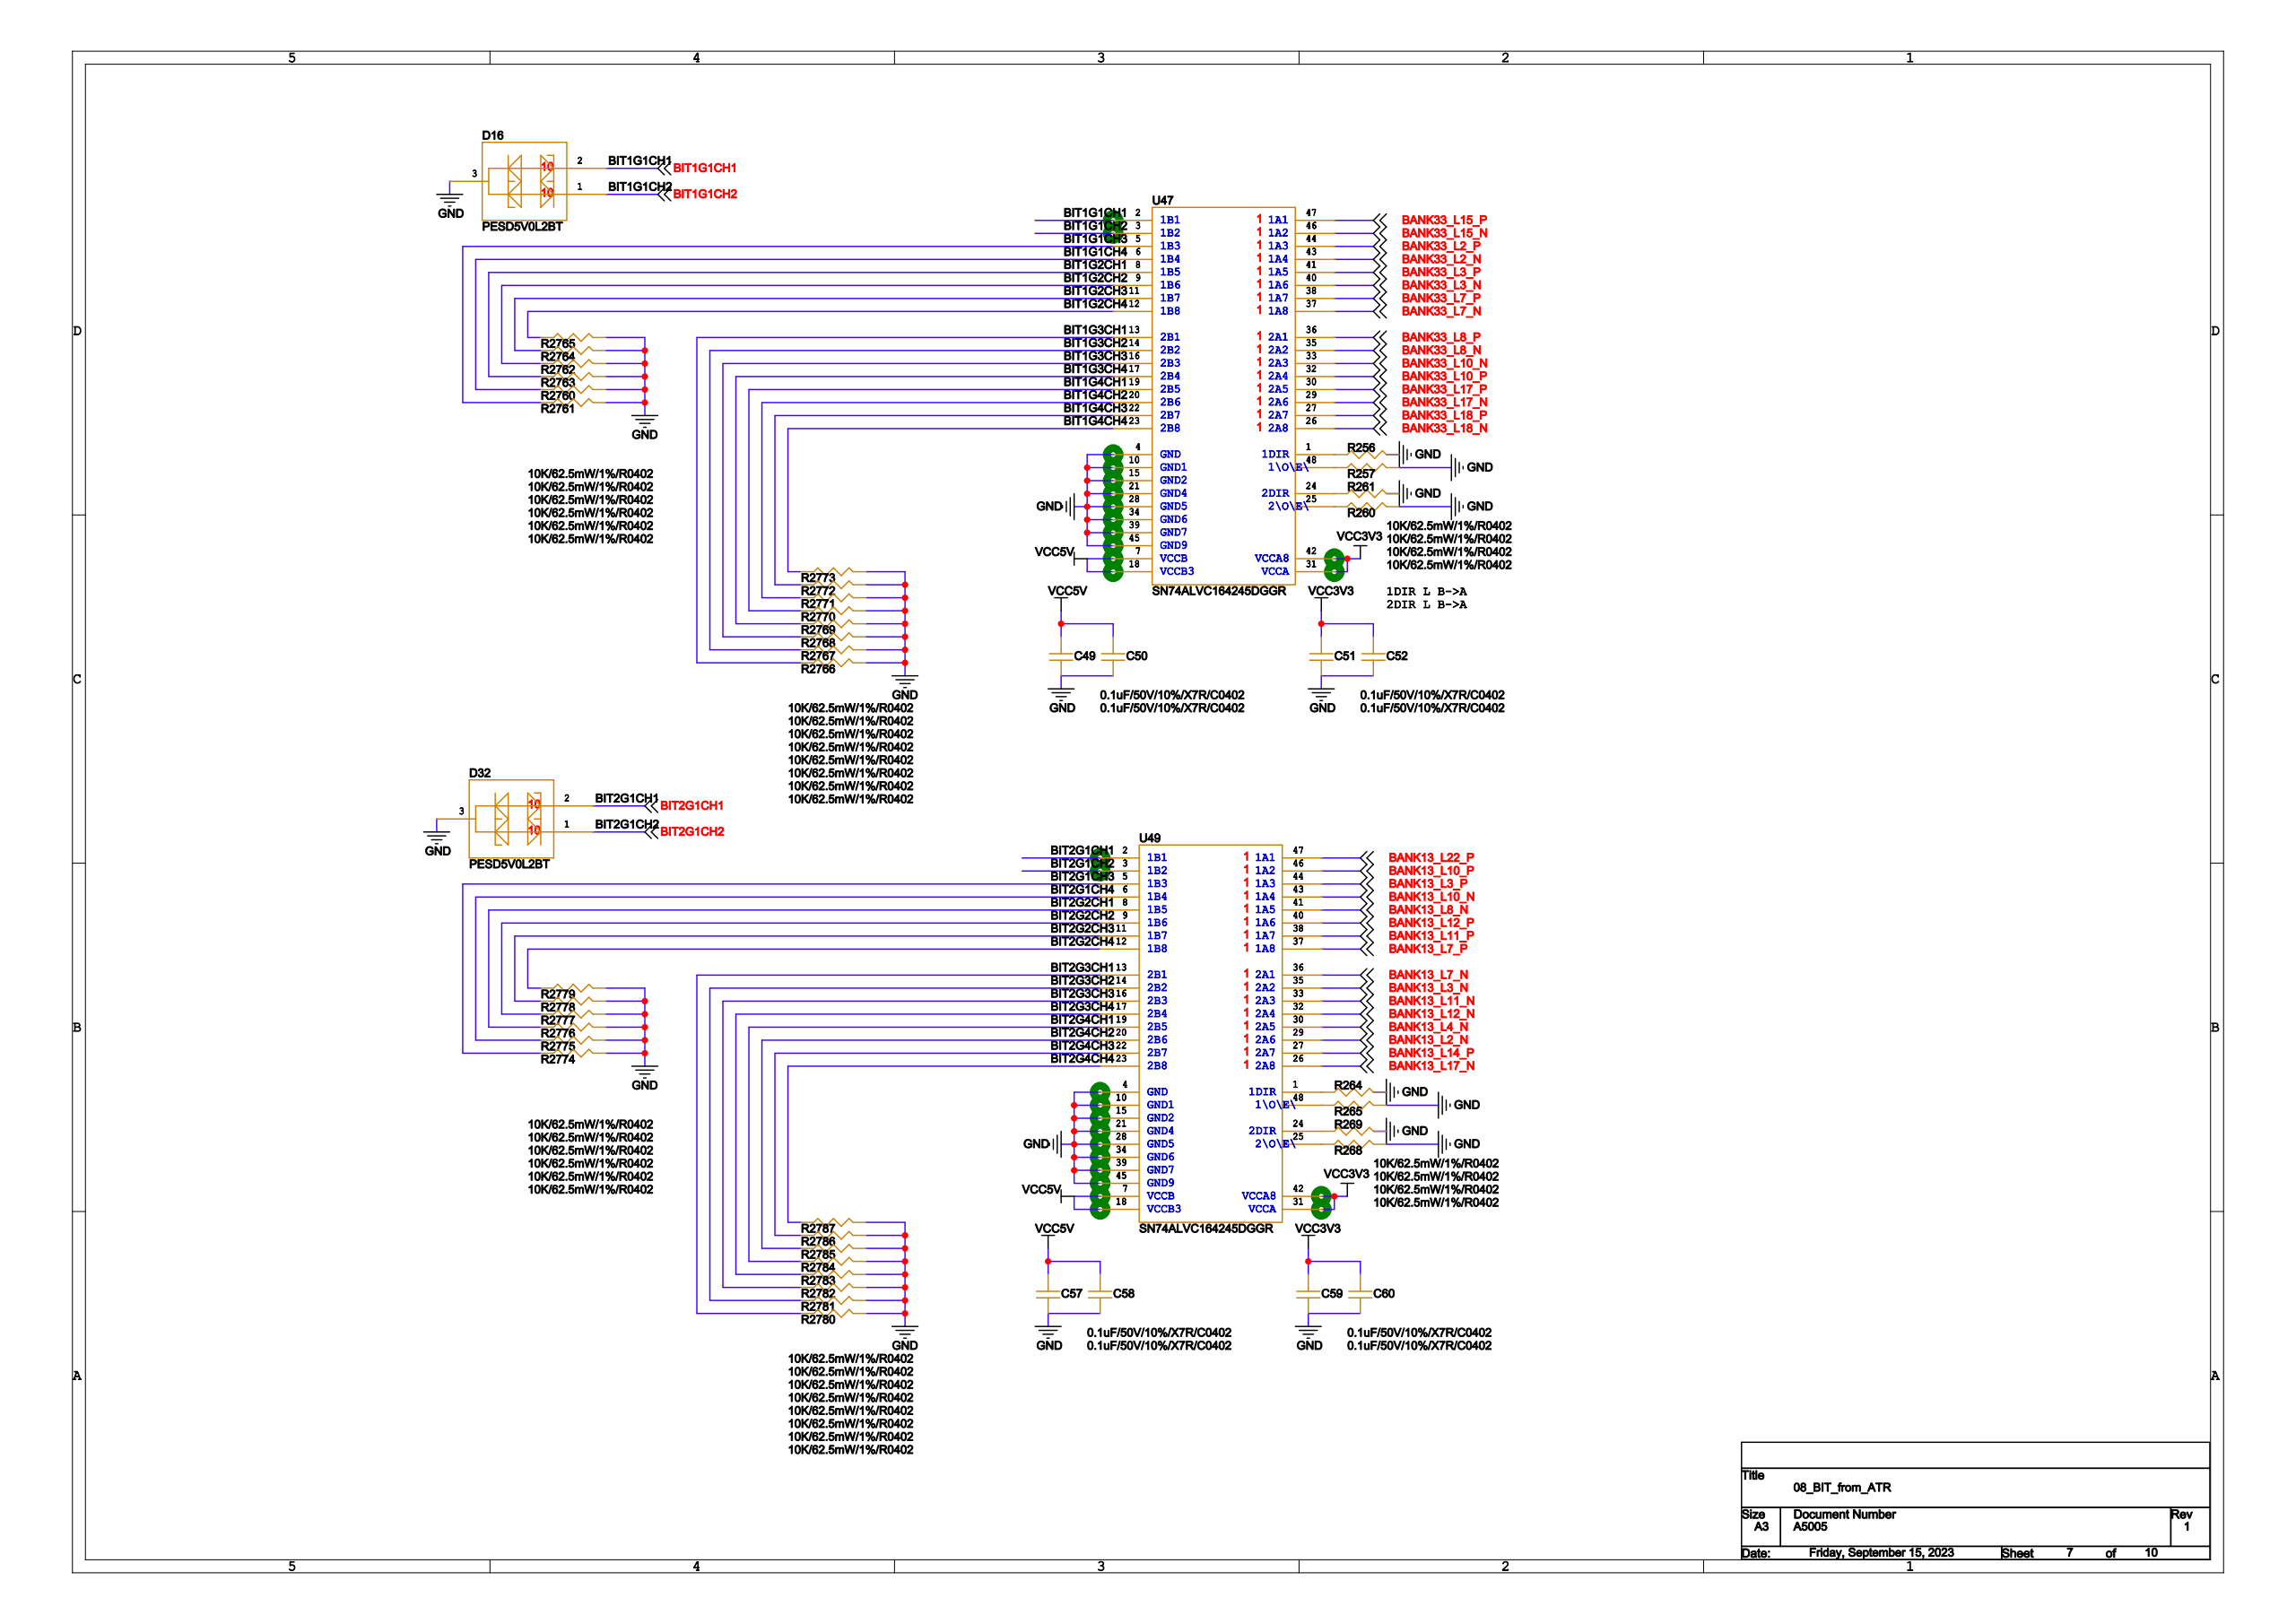Circuit board | Cadence Allegro | 634 parts | 645 nets | one sheet of the schematic
Parts on this sheet (reference | value | footprint):
C49 | 0.1uF/50V/10%/X7R/C0402 | 0402
C50 | 0.1uF/50V/10%/X7R/C0402 | 0402
C51 | 0.1uF/50V/10%/X7R/C0402 | 0402
C52 | 0.1uF/50V/10%/X7R/C0402 | 0402
C57 | 0.1uF/50V/10%/X7R/C0402 | 0402
C58 | 0.1uF/50V/10%/X7R/C0402 | 0402
C59 | 0.1uF/50V/10%/X7R/C0402 | 0402
C60 | 0.1uF/50V/10%/X7R/C0402 | 0402
D16 | PESD5V0L2BT | SOT23
D32 | PESD5V0L2BT | SOT23
R256 | 10K/62.5mW/1%/R0402 | 0402
R257 | 10K/62.5mW/1%/R0402 | 0402
R260 | 10K/62.5mW/1%/R0402 | 0402
R261 | 10K/62.5mW/1%/R0402 | 0402
R264 | 10K/62.5mW/1%/R0402 | 0402
R265 | 10K/62.5mW/1%/R0402 | 0402
R268 | 10K/62.5mW/1%/R0402 | 0402
R269 | 10K/62.5mW/1%/R0402 | 0402
R2760 | 10K/62.5mW/1%/R0402 | 0402
R2761 | 10K/62.5mW/1%/R0402 | 0402
R2762 | 10K/62.5mW/1%/R0402 | 0402
R2763 | 10K/62.5mW/1%/R0402 | 0402
R2764 | 10K/62.5mW/1%/R0402 | 0402
R2765 | 10K/62.5mW/1%/R0402 | 0402
R2766 | 10K/62.5mW/1%/R0402 | 0402
R2767 | 10K/62.5mW/1%/R0402 | 0402
R2768 | 10K/62.5mW/1%/R0402 | 0402
R2769 | 10K/62.5mW/1%/R0402 | 0402
R2770 | 10K/62.5mW/1%/R0402 | 0402
R2771 | 10K/62.5mW/1%/R0402 | 0402
R2772 | 10K/62.5mW/1%/R0402 | 0402
R2773 | 10K/62.5mW/1%/R0402 | 0402
R2774 | 10K/62.5mW/1%/R0402 | 0402
R2775 | 10K/62.5mW/1%/R0402 | 0402
R2776 | 10K/62.5mW/1%/R0402 | 0402
R2777 | 10K/62.5mW/1%/R0402 | 0402
R2778 | 10K/62.5mW/1%/R0402 | 0402
R2779 | 10K/62.5mW/1%/R0402 | 0402
R2780 | 10K/62.5mW/1%/R0402 | 0402
R2781 | 10K/62.5mW/1%/R0402 | 0402
R2782 | 10K/62.5mW/1%/R0402 | 0402
R2783 | 10K/62.5mW/1%/R0402 | 0402
R2784 | 10K/62.5mW/1%/R0402 | 0402
R2785 | 10K/62.5mW/1%/R0402 | 0402
R2786 | 10K/62.5mW/1%/R0402 | 0402
R2787 | 10K/62.5mW/1%/R0402 | 0402
U47 | SN74ALVC164245DGGR | TSSOP-48
U49 | SN74ALVC164245DGGR | TSSOP-48
Nets of these parts (net: part-pin ...):
AGND: C49-1 C50-1 C51-1 C52-1 C57-1 C58-1 C59-1 C60-1 D16-3 D32-3 R256-1 R257-1 R260-1 R261-1 R264-1 R265-1 R268-1 R269-1 R2760-1 R2761-1 R2762-1 R2763-1 R2764-1 R2765-1 R2766-1 R2767-1 R2768-1 R2769-1 R2770-1 R2771-1 R2772-1 R2773-1 R2774-1 R2775-1 R2776-1 R2777-1 R2778-1 R2779-1 R2780-1 R2781-1 R2782-1 R2783-1 R2784-1 R2785-1 R2786-1 R2787-1 U47-4 U47-10 U47-15 U47-21 U47-28 U47-34 U47-39 U47-45 U49-4 U49-10 U49-15 U49-21 U49-28 U49-34 U49-39 U49-45
BANK13_L8_N: U49-41
BANK13_L12_P: U49-40
BANK13_L11_P: U49-38
BANK13_L7_P: U49-37
BANK13_L7_N: U49-36
BANK13_L3_N: U49-35
BANK13_L11_N: U49-33
BANK13_L12_N: U49-32
BANK13_L4_N: U49-30
BANK13_L2_N: U49-29
BANK13_L14_P: U49-27
BANK13_L17_N: U49-26
3.3V: C51-2 C52-2 C59-2 C60-2 U47-31 U47-42 U49-31 U49-42
BANK13_L22_P: U49-47
BANK13_L10_P: U49-46
BANK13_L3_P: U49-44
BANK13_L10_N: U49-43
BANK33_L18_N: U47-26
BANK33_L18_P: U47-27
BANK33_L15_P: U47-47
BANK33_L17_N: U47-29
BANK33_L15_N: U47-46
BANK33_L17_P: U47-30
BANK33_L2_P: U47-44
BANK33_L10_P: U47-32
BANK33_L2_N: U47-43
BANK33_L10_N: U47-33
BANK33_L3_P: U47-41
BANK33_L8_N: U47-35
BANK33_L3_N: U47-40
BANK33_L7_N: U47-37
BANK33_L7_P: U47-38
BANK33_L8_P: U47-36
VCC5V: C49-2 C50-2 C57-2 C58-2 U47-7 U47-18 U49-7 U49-18
BIT1G1CH1: D16-2 U47-2
BIT2G1CH1: D32-2 U49-2
BIT1G1CH2: D16-1 U47-3
BIT2G1CH2: D32-1 U49-3
BIT1G1CH4: R2760-2 U47-6
BIT1G1CH3: R2761-2 U47-5
BIT1G2CH2: R2762-2 U47-9
BIT1G2CH1: R2763-2 U47-8
BIT1G2CH3: R2764-2 U47-11
BIT1G2CH4: R2765-2 U47-12
BIT1G3CH1: R2766-2 U47-13
BIT1G3CH2: R2767-2 U47-14
BIT1G3CH3: R2768-2 U47-16
BIT1G3CH4: R2769-2 U47-17
BIT1G4CH1: R2770-2 U47-19
BIT1G4CH2: R2771-2 U47-20
BIT1G4CH3: R2772-2 U47-22
BIT1G4CH4: R2773-2 U47-23
BIT2G1CH3: R2774-2 U49-5
BIT2G1CH4: R2775-2 U49-6
BIT2G2CH1: R2776-2 U49-8
BIT2G2CH2: R2777-2 U49-9
BIT2G2CH3: R2778-2 U49-11
BIT2G2CH4: R2779-2 U49-12
BIT2G3CH1: R2780-2 U49-13
BIT2G3CH2: R2781-2 U49-14
BIT2G3CH3: R2782-2 U49-16
BIT2G3CH4: R2783-2 U49-17
BIT2G4CH1: R2784-2 U49-19
BIT2G4CH2: R2785-2 U49-20
BIT2G4CH3: R2786-2 U49-22
BIT2G4CH4: R2787-2 U49-23
N240386151: R256-2 U47-1
N2403877347: R257-2
N240386071: R260-2
N240385751: R261-2 U47-24
N240482211: R264-2 U49-1
N2404837947: R265-2
N240482131: R268-2
N240481811: R269-2 U49-24